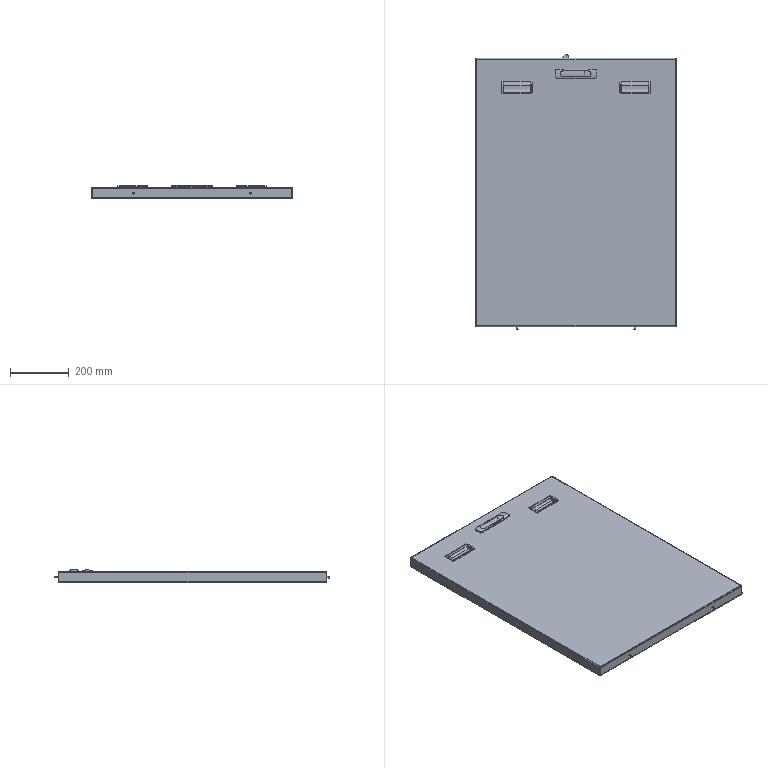Part | SolidWorks | 6 solids | 488 faces | box 685 x 936.5 x 44 mm | volume 1322747 mm3 | plane 222 | cylinder 188 | spline 46 | cone 26 | torus 6 | commonest cylinder face diameters 10 x27 2 x20 8.136 x15 6.6 x12 7 x11 3.242 x8